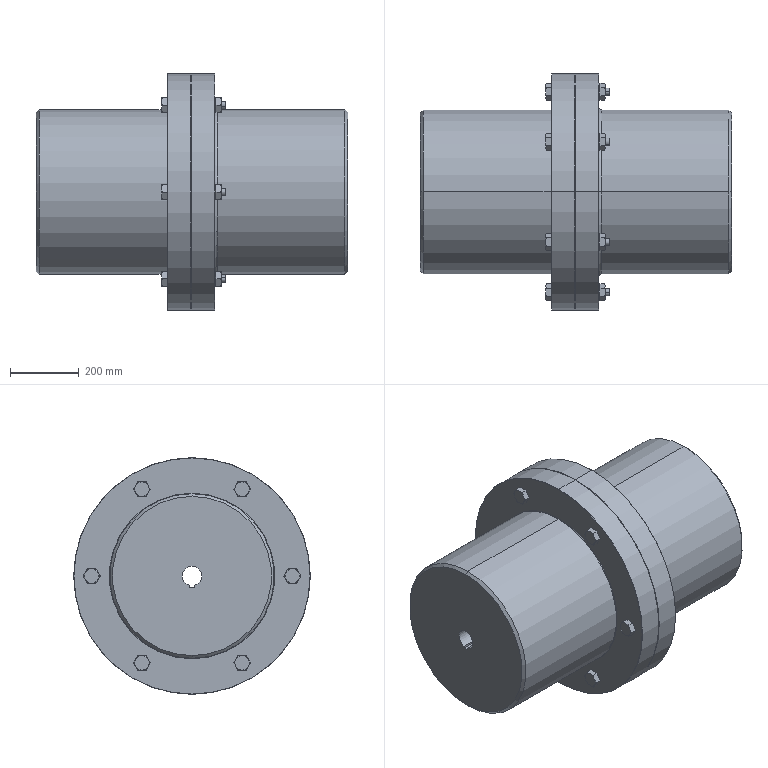Part | SolidWorks | features ICE 15, Chamfer 6, Revolution 3, CirPattern 2, Fillet 2, Scale 1 | 1 solid | 433 faces | box 907.5 x 690 x 690 mm | volume 187039199 mm3 | plane 223 | cone 144 | cylinder 62 | torus 4 | commonest cylinder face diameters 21 x36 42 x12 480 x7 690 x4 57 x3